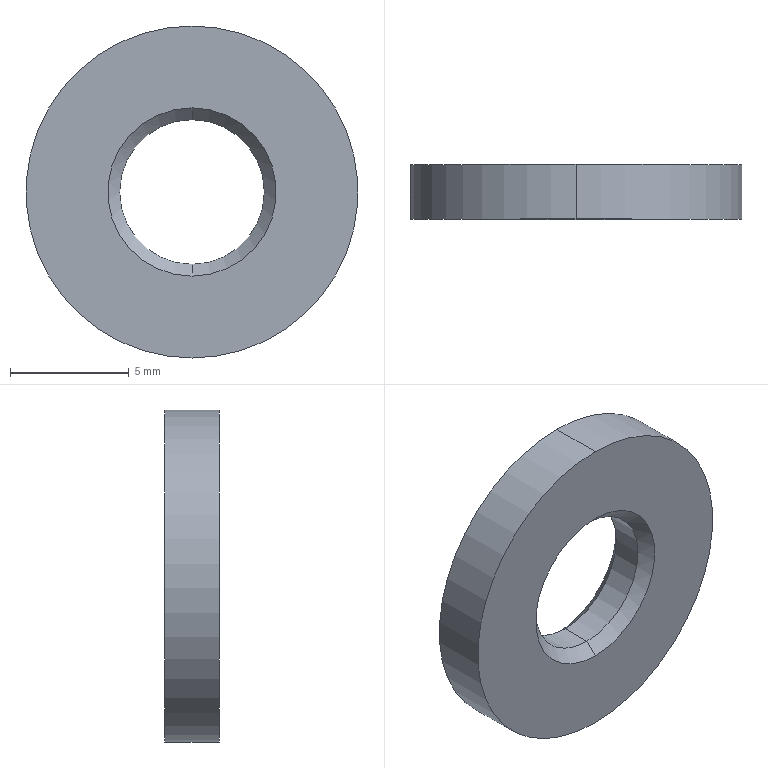Part | SolidWorks | features Chamfer 1, FlatPattern 1, SMBaseFlange 1, SheetMetal 1 | 1 solid | 10 faces | box 14 x 2.3 x 14 mm | volume 281.788 mm3 | cone 4 | cylinder 4 | plane 2 | commonest cylinder face diameters 6.1 x2 14 x2
STEP:
#1=CARTESIAN_POINT('',(0.,-0.5,-3.05));
#2=VERTEX_POINT('',#1);
#3=CARTESIAN_POINT('',(0.,-0.5,3.05));
#4=VERTEX_POINT('',#3);
#5=CARTESIAN_POINT('',(0.,-0.5,0.));
#6=DIRECTION('',(0.,1.,0.));
#7=DIRECTION('',(0.,0.,1.));
#8=AXIS2_PLACEMENT_3D('',#5,#6,#7);
#9=CIRCLE('',#8,3.05);
#10=EDGE_CURVE('',#2,#4,#9,.T.);
#11=ORIENTED_EDGE('',*,*,#10,.F.);
#12=CARTESIAN_POINT('',(0.,0.,-3.55));
#13=VERTEX_POINT('',#12);
#14=CARTESIAN_POINT('',(0.,-0.5,-3.05));
#15=DIRECTION('',(0.,0.7071,-0.7071));
#16=VECTOR('',#15,1000.);
#17=LINE('',#14,#16);
#18=EDGE_CURVE('',#2,#13,#17,.T.);
#19=ORIENTED_EDGE('',*,*,#18,.T.);
#20=CARTESIAN_POINT('',(0.,0.,3.55));
#21=VERTEX_POINT('',#20);
#22=CARTESIAN_POINT('',(0.,0.,0.));
#23=DIRECTION('',(0.,-1.,0.));
#24=DIRECTION('',(0.,0.,1.));
#25=AXIS2_PLACEMENT_3D('',#22,#23,#24);
#26=CIRCLE('',#25,3.55);
#27=EDGE_CURVE('',#21,#13,#26,.T.);
#28=ORIENTED_EDGE('',*,*,#27,.F.);
#29=CARTESIAN_POINT('',(0.,-0.5,3.05));
#30=DIRECTION('',(0.,0.7071,0.7071));
#31=VECTOR('',#30,1000.);
#32=LINE('',#29,#31);
#33=EDGE_CURVE('',#4,#21,#32,.T.);
#34=ORIENTED_EDGE('',*,*,#33,.F.);
#35=EDGE_LOOP('',(#11,#19,#28,#34));
#36=FACE_OUTER_BOUND('',#35,.T.);
#37=CARTESIAN_POINT('',(0.,-0.5,0.));
#38=DIRECTION('',(0.,1.,0.));
#39=DIRECTION('',(0.,0.,1.));
#40=AXIS2_PLACEMENT_3D('',#37,#38,#39);
#41=CONICAL_SURFACE('',#40,3.05,0.7854);
#42=ADVANCED_FACE('',(#36),#41,.F.);
#43=CARTESIAN_POINT('',(0.,-1.8,3.05));
#44=VERTEX_POINT('',#43);
#45=CARTESIAN_POINT('',(0.,-1.8,-3.05));
#46=VERTEX_POINT('',#45);
#47=CARTESIAN_POINT('',(0.,-1.8,0.));
#48=DIRECTION('',(0.,-1.,0.));
#49=DIRECTION('',(0.,0.,1.));
#50=AXIS2_PLACEMENT_3D('',#47,#48,#49);
#51=CIRCLE('',#50,3.05);
#52=EDGE_CURVE('',#44,#46,#51,.T.);
#53=ORIENTED_EDGE('',*,*,#52,.F.);
#54=CARTESIAN_POINT('',(0.,-2.3,3.55));
#55=VERTEX_POINT('',#54);
#56=CARTESIAN_POINT('',(0.,-2.3,3.55));
#57=DIRECTION('',(0.,-0.7071,0.7071));
#58=VECTOR('',#57,1000.);
#59=LINE('',#56,#58);
#60=EDGE_CURVE('',#44,#55,#59,.T.);
#61=ORIENTED_EDGE('',*,*,#60,.T.);
#62=CARTESIAN_POINT('',(0.,-2.3,-3.55));
#63=VERTEX_POINT('',#62);
#64=CARTESIAN_POINT('',(0.,-2.3,0.));
#65=DIRECTION('',(0.,1.,0.));
#66=DIRECTION('',(0.,0.,1.));
#67=AXIS2_PLACEMENT_3D('',#64,#65,#66);
#68=CIRCLE('',#67,3.55);
#69=EDGE_CURVE('',#63,#55,#68,.T.);
#70=ORIENTED_EDGE('',*,*,#69,.F.);
#71=CARTESIAN_POINT('',(0.,-2.3,-3.55));
#72=DIRECTION('',(0.,-0.7071,-0.7071));
#73=VECTOR('',#72,1000.);
#74=LINE('',#71,#73);
#75=EDGE_CURVE('',#46,#63,#74,.T.);
#76=ORIENTED_EDGE('',*,*,#75,.F.);
#77=EDGE_LOOP('',(#53,#61,#70,#76));
#78=FACE_OUTER_BOUND('',#77,.T.);
#79=CARTESIAN_POINT('',(0.,-2.3,0.));
#80=DIRECTION('',(0.,-1.,0.));
#81=DIRECTION('',(0.,0.,-1.));
#82=AXIS2_PLACEMENT_3D('',#79,#80,#81);
#83=CONICAL_SURFACE('',#82,3.55,0.7854);
#84=ADVANCED_FACE('',(#78),#83,.F.);
#85=ORIENTED_EDGE('',*,*,#52,.T.);
#86=CARTESIAN_POINT('',(0.,-2.3,-3.05));
#87=DIRECTION('',(0.,1.,0.));
#88=VECTOR('',#87,1000.);
#89=LINE('',#86,#88);
#90=EDGE_CURVE('',#46,#2,#89,.T.);
#91=ORIENTED_EDGE('',*,*,#90,.T.);
#92=ORIENTED_EDGE('',*,*,#10,.T.);
#93=CARTESIAN_POINT('',(0.,-2.3,3.05));
#94=DIRECTION('',(0.,1.,0.));
#95=VECTOR('',#94,1000.);
#96=LINE('',#93,#95);
#97=EDGE_CURVE('',#44,#4,#96,.T.);
#98=ORIENTED_EDGE('',*,*,#97,.F.);
#99=EDGE_LOOP('',(#85,#91,#92,#98));
#100=FACE_OUTER_BOUND('',#99,.T.);
#101=CARTESIAN_POINT('',(0.,-2.3,0.));
#102=DIRECTION('',(0.,1.,0.));
#103=DIRECTION('',(0.,0.,1.));
#104=AXIS2_PLACEMENT_3D('',#101,#102,#103);
#105=CYLINDRICAL_SURFACE('',#104,3.05);
#106=ADVANCED_FACE('',(#100),#105,.F.);
#107=CARTESIAN_POINT('',(0.,-2.3,7.));
#108=VERTEX_POINT('',#107);
#109=CARTESIAN_POINT('',(0.,-2.3,-7.));
#110=VERTEX_POINT('',#109);
#111=CARTESIAN_POINT('',(0.,-2.3,0.));
#112=DIRECTION('',(0.,1.,0.));
#113=DIRECTION('',(0.,0.,1.));
#114=AXIS2_PLACEMENT_3D('',#111,#112,#113);
#115=CIRCLE('',#114,7.);
#116=EDGE_CURVE('',#108,#110,#115,.T.);
#117=ORIENTED_EDGE('',*,*,#116,.T.);
#118=CARTESIAN_POINT('',(0.,0.,-7.));
#119=VERTEX_POINT('',#118);
#120=CARTESIAN_POINT('',(0.,-2.3,-7.));
#121=DIRECTION('',(0.,1.,0.));
#122=VECTOR('',#121,1000.);
#123=LINE('',#120,#122);
#124=EDGE_CURVE('',#110,#119,#123,.T.);
#125=ORIENTED_EDGE('',*,*,#124,.T.);
#126=CARTESIAN_POINT('',(0.,0.,7.));
#127=VERTEX_POINT('',#126);
#128=CARTESIAN_POINT('',(0.,0.,0.));
#129=DIRECTION('',(0.,1.,0.));
#130=DIRECTION('',(0.,0.,1.));
#131=AXIS2_PLACEMENT_3D('',#128,#129,#130);
#132=CIRCLE('',#131,7.);
#133=EDGE_CURVE('',#127,#119,#132,.T.);
#134=ORIENTED_EDGE('',*,*,#133,.F.);
#135=CARTESIAN_POINT('',(0.,-2.3,7.));
#136=DIRECTION('',(0.,1.,0.));
#137=VECTOR('',#136,1000.);
#138=LINE('',#135,#137);
#139=EDGE_CURVE('',#108,#127,#138,.T.);
#140=ORIENTED_EDGE('',*,*,#139,.F.);
#141=EDGE_LOOP('',(#117,#125,#134,#140));
#142=FACE_OUTER_BOUND('',#141,.T.);
#143=CARTESIAN_POINT('',(0.,-2.3,0.));
#144=DIRECTION('',(0.,1.,0.));
#145=DIRECTION('',(0.,0.,1.));
#146=AXIS2_PLACEMENT_3D('',#143,#144,#145);
#147=CYLINDRICAL_SURFACE('',#146,7.);
#148=ADVANCED_FACE('',(#142),#147,.T.);
#149=ORIENTED_EDGE('',*,*,#124,.F.);
#150=CARTESIAN_POINT('',(0.,-2.3,0.));
#151=DIRECTION('',(0.,1.,0.));
#152=DIRECTION('',(0.,0.,1.));
#153=AXIS2_PLACEMENT_3D('',#150,#151,#152);
#154=CIRCLE('',#153,7.);
#155=EDGE_CURVE('',#110,#108,#154,.T.);
#156=ORIENTED_EDGE('',*,*,#155,.T.);
#157=ORIENTED_EDGE('',*,*,#139,.T.);
#158=CARTESIAN_POINT('',(0.,0.,0.));
#159=DIRECTION('',(0.,1.,0.));
#160=DIRECTION('',(0.,0.,1.));
#161=AXIS2_PLACEMENT_3D('',#158,#159,#160);
#162=CIRCLE('',#161,7.);
#163=EDGE_CURVE('',#119,#127,#162,.T.);
#164=ORIENTED_EDGE('',*,*,#163,.F.);
#165=EDGE_LOOP('',(#149,#156,#157,#164));
#166=FACE_OUTER_BOUND('',#165,.T.);
#167=CARTESIAN_POINT('',(0.,-2.3,0.));
#168=DIRECTION('',(0.,1.,0.));
#169=DIRECTION('',(0.,0.,1.));
#170=AXIS2_PLACEMENT_3D('',#167,#168,#169);
#171=CYLINDRICAL_SURFACE('',#170,7.);
#172=ADVANCED_FACE('',(#166),#171,.T.);
#173=ORIENTED_EDGE('',*,*,#69,.T.);
#174=CARTESIAN_POINT('',(0.,-2.3,0.));
#175=DIRECTION('',(0.,1.,0.));
#176=DIRECTION('',(0.,0.,1.));
#177=AXIS2_PLACEMENT_3D('',#174,#175,#176);
#178=CIRCLE('',#177,3.55);
#179=EDGE_CURVE('',#55,#63,#178,.T.);
#180=ORIENTED_EDGE('',*,*,#179,.T.);
#181=EDGE_LOOP('',(#173,#180));
#182=FACE_BOUND('',#181,.T.);
#183=ORIENTED_EDGE('',*,*,#116,.F.);
#184=ORIENTED_EDGE('',*,*,#155,.F.);
#185=EDGE_LOOP('',(#183,#184));
#186=FACE_OUTER_BOUND('',#185,.T.);
#187=CARTESIAN_POINT('',(0.,-2.3,0.));
#188=DIRECTION('',(0.,1.,0.));
#189=DIRECTION('',(0.,0.,1.));
#190=AXIS2_PLACEMENT_3D('',#187,#188,#189);
#191=PLANE('',#190);
#192=ADVANCED_FACE('',(#182,#186),#191,.F.);
#193=ORIENTED_EDGE('',*,*,#27,.T.);
#194=CARTESIAN_POINT('',(0.,0.,0.));
#195=DIRECTION('',(0.,-1.,0.));
#196=DIRECTION('',(0.,0.,1.));
#197=AXIS2_PLACEMENT_3D('',#194,#195,#196);
#198=CIRCLE('',#197,3.55);
#199=EDGE_CURVE('',#13,#21,#198,.T.);
#200=ORIENTED_EDGE('',*,*,#199,.T.);
#201=EDGE_LOOP('',(#193,#200));
#202=FACE_BOUND('',#201,.T.);
#203=ORIENTED_EDGE('',*,*,#133,.T.);
#204=ORIENTED_EDGE('',*,*,#163,.T.);
#205=EDGE_LOOP('',(#203,#204));
#206=FACE_OUTER_BOUND('',#205,.T.);
#207=CARTESIAN_POINT('',(0.,0.,0.));
#208=DIRECTION('',(0.,1.,0.));
#209=DIRECTION('',(0.,0.,1.));
#210=AXIS2_PLACEMENT_3D('',#207,#208,#209);
#211=PLANE('',#210);
#212=ADVANCED_FACE('',(#202,#206),#211,.T.);
#213=ORIENTED_EDGE('',*,*,#90,.F.);
#214=CARTESIAN_POINT('',(0.,-1.8,0.));
#215=DIRECTION('',(0.,-1.,0.));
#216=DIRECTION('',(0.,0.,1.));
#217=AXIS2_PLACEMENT_3D('',#214,#215,#216);
#218=CIRCLE('',#217,3.05);
#219=EDGE_CURVE('',#46,#44,#218,.T.);
#220=ORIENTED_EDGE('',*,*,#219,.T.);
#221=ORIENTED_EDGE('',*,*,#97,.T.);
#222=CARTESIAN_POINT('',(0.,-0.5,0.));
#223=DIRECTION('',(0.,1.,0.));
#224=DIRECTION('',(0.,0.,1.));
#225=AXIS2_PLACEMENT_3D('',#222,#223,#224);
#226=CIRCLE('',#225,3.05);
#227=EDGE_CURVE('',#4,#2,#226,.T.);
#228=ORIENTED_EDGE('',*,*,#227,.T.);
#229=EDGE_LOOP('',(#213,#220,#221,#228));
#230=FACE_OUTER_BOUND('',#229,.T.);
#231=CARTESIAN_POINT('',(0.,-2.3,0.));
#232=DIRECTION('',(0.,1.,0.));
#233=DIRECTION('',(0.,0.,1.));
#234=AXIS2_PLACEMENT_3D('',#231,#232,#233);
#235=CYLINDRICAL_SURFACE('',#234,3.05);
#236=ADVANCED_FACE('',(#230),#235,.F.);
#237=ORIENTED_EDGE('',*,*,#60,.F.);
#238=ORIENTED_EDGE('',*,*,#219,.F.);
#239=ORIENTED_EDGE('',*,*,#75,.T.);
#240=ORIENTED_EDGE('',*,*,#179,.F.);
#241=EDGE_LOOP('',(#237,#238,#239,#240));
#242=FACE_OUTER_BOUND('',#241,.T.);
#243=CARTESIAN_POINT('',(0.,-2.3,0.));
#244=DIRECTION('',(0.,-1.,0.));
#245=DIRECTION('',(0.,0.,-1.));
#246=AXIS2_PLACEMENT_3D('',#243,#244,#245);
#247=CONICAL_SURFACE('',#246,3.55,0.7854);
#248=ADVANCED_FACE('',(#242),#247,.F.);
#249=ORIENTED_EDGE('',*,*,#18,.F.);
#250=ORIENTED_EDGE('',*,*,#227,.F.);
#251=ORIENTED_EDGE('',*,*,#33,.T.);
#252=ORIENTED_EDGE('',*,*,#199,.F.);
#253=EDGE_LOOP('',(#249,#250,#251,#252));
#254=FACE_OUTER_BOUND('',#253,.T.);
#255=CARTESIAN_POINT('',(0.,-0.5,0.));
#256=DIRECTION('',(0.,1.,0.));
#257=DIRECTION('',(0.,0.,1.));
#258=AXIS2_PLACEMENT_3D('',#255,#256,#257);
#259=CONICAL_SURFACE('',#258,3.05,0.7854);
#260=ADVANCED_FACE('',(#254),#259,.F.);
#261=CLOSED_SHELL('',(#42,#84,#106,#148,#172,#192,#212,#236,#248,#260));
#262=MANIFOLD_SOLID_BREP('',#261);
#263=CARTESIAN_POINT('',(0.,0.,0.));
#264=DIRECTION('',(0.,0.,1.));
#265=DIRECTION('',(1.,0.,0.));
#266=AXIS2_PLACEMENT_3D('',#263,#264,#265);
#267=(LENGTH_UNIT()NAMED_UNIT(*)SI_UNIT(.MILLI.,.METRE.));
#268=UNCERTAINTY_MEASURE_WITH_UNIT(LENGTH_MEASURE(0.00001),#267,'','');
#269=(NAMED_UNIT(*)PLANE_ANGLE_UNIT()SI_UNIT($,.RADIAN.));
#270=(NAMED_UNIT(*)SI_UNIT($,.STERADIAN.)SOLID_ANGLE_UNIT());
#271=(GEOMETRIC_REPRESENTATION_CONTEXT(3)GLOBAL_UNCERTAINTY_ASSIGNED_CONTEXT((#268))GLOBAL_UNIT_ASSIGNED_CONTEXT((#267,#269,#270))REPRESENTATION_CONTEXT('',''));
#272=ADVANCED_BREP_SHAPE_REPRESENTATION('',(#262,#266),#271);